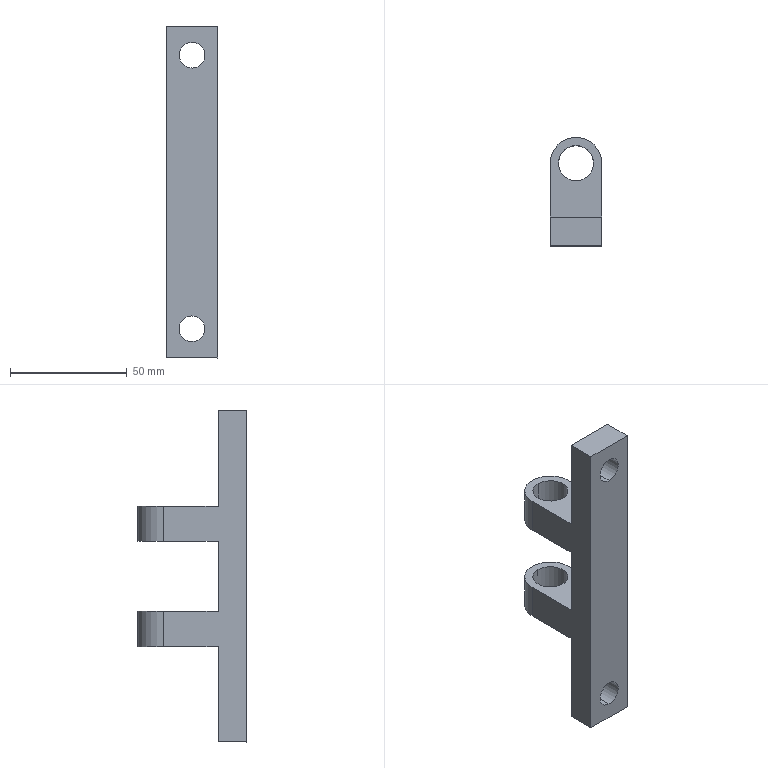Part | SolidWorks | features BaseBody 1 | 1 solid | 22 faces | box 22.041 x 46.517 x 142.008 mm | volume 51119 mm3 | plane 12 | cylinder 10 | commonest cylinder face diameters 11 x4 15 x4 22 x2
STEP:
#1=CARTESIAN_POINT('',(406.066,-39.21,30.764));
#2=VERTEX_POINT('',#1);
#3=CARTESIAN_POINT('',(406.062,-39.209,19.764));
#4=VERTEX_POINT('',#3);
#5=CARTESIAN_POINT('',(406.064,-39.21,25.264));
#6=DIRECTION('',(-0.000000041,-1.,-0.0001428));
#7=DIRECTION('',(-0.0001431,0.0001428,-1.));
#8=AXIS2_PLACEMENT_3D('',#5,#6,#7);
#9=CIRCLE('',#8,5.5);
#10=EDGE_CURVE('',#2,#4,#9,.T.);
#11=ORIENTED_EDGE('',*,*,#10,.F.);
#12=CARTESIAN_POINT('',(406.066,-51.21,30.763));
#13=VERTEX_POINT('',#12);
#14=CARTESIAN_POINT('',(406.066,-51.212,30.763));
#15=DIRECTION('',(-0.000000041,-1.,-0.0001428));
#16=VECTOR('',#15,1000.);
#17=LINE('',#14,#16);
#18=EDGE_CURVE('',#2,#13,#17,.T.);
#19=ORIENTED_EDGE('',*,*,#18,.T.);
#20=CARTESIAN_POINT('',(406.062,-51.209,19.763));
#21=VERTEX_POINT('',#20);
#22=CARTESIAN_POINT('',(406.064,-51.21,25.263));
#23=DIRECTION('',(0.000000041,1.,0.0001428));
#24=DIRECTION('',(-0.0002857,0.0001428,-1.));
#25=AXIS2_PLACEMENT_3D('',#22,#23,#24);
#26=CIRCLE('',#25,5.5);
#27=EDGE_CURVE('',#21,#13,#26,.T.);
#28=ORIENTED_EDGE('',*,*,#27,.F.);
#29=CARTESIAN_POINT('',(406.062,-51.21,19.763));
#30=DIRECTION('',(-0.000000041,-1.,-0.0001428));
#31=VECTOR('',#30,1000.);
#32=LINE('',#29,#31);
#33=EDGE_CURVE('',#4,#21,#32,.T.);
#34=ORIENTED_EDGE('',*,*,#33,.F.);
#35=EDGE_LOOP('',(#11,#19,#28,#34));
#36=FACE_OUTER_BOUND('',#35,.T.);
#37=CARTESIAN_POINT('',(406.064,-51.211,25.263));
#38=DIRECTION('',(-0.000000041,-1.,-0.0001428));
#39=DIRECTION('',(-0.0002857,0.0001428,-1.));
#40=AXIS2_PLACEMENT_3D('',#37,#38,#39);
#41=CYLINDRICAL_SURFACE('',#40,5.5);
#42=ADVANCED_FACE('',(#36),#41,.F.);
#43=CARTESIAN_POINT('',(406.069,-8.211,53.586));
#44=VERTEX_POINT('',#43);
#45=CARTESIAN_POINT('',(406.069,-23.211,53.584));
#46=VERTEX_POINT('',#45);
#47=CARTESIAN_POINT('',(406.069,-15.711,53.585));
#48=DIRECTION('',(0.0002857,-0.0001428,1.));
#49=DIRECTION('',(-0.000000041,-1.,-0.0001428));
#50=AXIS2_PLACEMENT_3D('',#47,#48,#49);
#51=CIRCLE('',#50,7.5);
#52=EDGE_CURVE('',#44,#46,#51,.T.);
#53=ORIENTED_EDGE('',*,*,#52,.F.);
#54=CARTESIAN_POINT('',(406.073,-8.213,68.586));
#55=VERTEX_POINT('',#54);
#56=CARTESIAN_POINT('',(406.069,-8.211,53.586));
#57=DIRECTION('',(0.0002857,-0.0001428,1.));
#58=VECTOR('',#57,1000.);
#59=LINE('',#56,#58);
#60=EDGE_CURVE('',#44,#55,#59,.T.);
#61=ORIENTED_EDGE('',*,*,#60,.T.);
#62=CARTESIAN_POINT('',(406.073,-23.213,68.584));
#63=VERTEX_POINT('',#62);
#64=CARTESIAN_POINT('',(406.073,-15.713,68.585));
#65=DIRECTION('',(-0.0002857,0.0001428,-1.));
#66=DIRECTION('',(-0.000000041,-1.,-0.0001428));
#67=AXIS2_PLACEMENT_3D('',#64,#65,#66);
#68=CIRCLE('',#67,7.5);
#69=EDGE_CURVE('',#63,#55,#68,.T.);
#70=ORIENTED_EDGE('',*,*,#69,.F.);
#71=CARTESIAN_POINT('',(406.069,-23.211,53.584));
#72=DIRECTION('',(0.0002857,-0.0001428,1.));
#73=VECTOR('',#72,1000.);
#74=LINE('',#71,#73);
#75=EDGE_CURVE('',#46,#63,#74,.T.);
#76=ORIENTED_EDGE('',*,*,#75,.F.);
#77=EDGE_LOOP('',(#53,#61,#70,#76));
#78=FACE_OUTER_BOUND('',#77,.T.);
#79=CARTESIAN_POINT('',(406.069,-15.711,53.585));
#80=DIRECTION('',(0.0002857,-0.0001428,1.));
#81=DIRECTION('',(-0.000000041,-1.,-0.0001428));
#82=AXIS2_PLACEMENT_3D('',#79,#80,#81);
#83=CYLINDRICAL_SURFACE('',#82,7.5);
#84=ADVANCED_FACE('',(#78),#83,.F.);
#85=CARTESIAN_POINT('',(406.082,-8.218,98.586));
#86=VERTEX_POINT('',#85);
#87=CARTESIAN_POINT('',(406.082,-23.218,98.584));
#88=VERTEX_POINT('',#87);
#89=CARTESIAN_POINT('',(406.082,-15.718,98.585));
#90=DIRECTION('',(0.0002857,-0.0001428,1.));
#91=DIRECTION('',(0.000000041,1.,0.0001428));
#92=AXIS2_PLACEMENT_3D('',#89,#90,#91);
#93=CIRCLE('',#92,7.5);
#94=EDGE_CURVE('',#86,#88,#93,.T.);
#95=ORIENTED_EDGE('',*,*,#94,.F.);
#96=CARTESIAN_POINT('',(406.086,-8.22,113.586));
#97=VERTEX_POINT('',#96);
#98=CARTESIAN_POINT('',(406.069,-8.211,53.586));
#99=DIRECTION('',(0.0002857,-0.0001428,1.));
#100=VECTOR('',#99,1000.);
#101=LINE('',#98,#100);
#102=EDGE_CURVE('',#86,#97,#101,.T.);
#103=ORIENTED_EDGE('',*,*,#102,.T.);
#104=CARTESIAN_POINT('',(406.086,-23.22,113.584));
#105=VERTEX_POINT('',#104);
#106=CARTESIAN_POINT('',(406.086,-15.72,113.585));
#107=DIRECTION('',(-0.0002857,0.0001428,-1.));
#108=DIRECTION('',(0.000000041,1.,0.0001428));
#109=AXIS2_PLACEMENT_3D('',#106,#107,#108);
#110=CIRCLE('',#109,7.5);
#111=EDGE_CURVE('',#105,#97,#110,.T.);
#112=ORIENTED_EDGE('',*,*,#111,.F.);
#113=CARTESIAN_POINT('',(406.069,-23.211,53.584));
#114=DIRECTION('',(0.0002857,-0.0001428,1.));
#115=VECTOR('',#114,1000.);
#116=LINE('',#113,#115);
#117=EDGE_CURVE('',#88,#105,#116,.T.);
#118=ORIENTED_EDGE('',*,*,#117,.F.);
#119=EDGE_LOOP('',(#95,#103,#112,#118));
#120=FACE_OUTER_BOUND('',#119,.T.);
#121=CARTESIAN_POINT('',(406.069,-15.711,53.585));
#122=DIRECTION('',(0.0002857,-0.0001428,1.));
#123=DIRECTION('',(-0.000000041,-1.,-0.0001428));
#124=AXIS2_PLACEMENT_3D('',#121,#122,#123);
#125=CYLINDRICAL_SURFACE('',#124,7.5);
#126=ADVANCED_FACE('',(#120),#125,.F.);
#127=CARTESIAN_POINT('',(406.093,-39.227,147.764));
#128=VERTEX_POINT('',#127);
#129=CARTESIAN_POINT('',(406.089,-39.226,136.764));
#130=VERTEX_POINT('',#129);
#131=CARTESIAN_POINT('',(406.091,-39.226,142.264));
#132=DIRECTION('',(-0.000000041,-1.,-0.0001428));
#133=DIRECTION('',(-0.0001431,0.0001428,-1.));
#134=AXIS2_PLACEMENT_3D('',#131,#132,#133);
#135=CIRCLE('',#134,5.5);
#136=EDGE_CURVE('',#128,#130,#135,.T.);
#137=ORIENTED_EDGE('',*,*,#136,.F.);
#138=CARTESIAN_POINT('',(406.093,-51.227,147.763));
#139=VERTEX_POINT('',#138);
#140=CARTESIAN_POINT('',(406.093,-51.226,147.763));
#141=DIRECTION('',(-0.000000041,-1.,-0.0001428));
#142=VECTOR('',#141,1000.);
#143=LINE('',#140,#142);
#144=EDGE_CURVE('',#128,#139,#143,.T.);
#145=ORIENTED_EDGE('',*,*,#144,.T.);
#146=CARTESIAN_POINT('',(406.089,-51.226,136.763));
#147=VERTEX_POINT('',#146);
#148=CARTESIAN_POINT('',(406.091,-51.226,142.263));
#149=DIRECTION('',(0.000000041,1.,0.0001428));
#150=DIRECTION('',(-0.0002857,0.0001428,-1.));
#151=AXIS2_PLACEMENT_3D('',#148,#149,#150);
#152=CIRCLE('',#151,5.5);
#153=EDGE_CURVE('',#147,#139,#152,.T.);
#154=ORIENTED_EDGE('',*,*,#153,.F.);
#155=CARTESIAN_POINT('',(406.089,-51.224,136.763));
#156=DIRECTION('',(-0.000000041,-1.,-0.0001428));
#157=VECTOR('',#156,1000.);
#158=LINE('',#155,#157);
#159=EDGE_CURVE('',#130,#147,#158,.T.);
#160=ORIENTED_EDGE('',*,*,#159,.F.);
#161=EDGE_LOOP('',(#137,#145,#154,#160));
#162=FACE_OUTER_BOUND('',#161,.T.);
#163=CARTESIAN_POINT('',(406.091,-51.225,142.263));
#164=DIRECTION('',(-0.000000041,-1.,-0.0001428));
#165=DIRECTION('',(-0.0002857,0.0001428,-1.));
#166=AXIS2_PLACEMENT_3D('',#163,#164,#165);
#167=CYLINDRICAL_SURFACE('',#166,5.5);
#168=ADVANCED_FACE('',(#162),#167,.F.);
#169=CARTESIAN_POINT('',(417.057,-51.208,12.76));
#170=VERTEX_POINT('',#169);
#171=CARTESIAN_POINT('',(417.057,-39.208,12.761));
#172=VERTEX_POINT('',#171);
#173=CARTESIAN_POINT('',(417.057,-51.208,12.76));
#174=DIRECTION('',(0.000000041,1.,0.0001428));
#175=VECTOR('',#174,1000.);
#176=LINE('',#173,#175);
#177=EDGE_CURVE('',#170,#172,#176,.T.);
#178=ORIENTED_EDGE('',*,*,#177,.F.);
#179=CARTESIAN_POINT('',(395.057,-51.208,12.766));
#180=VERTEX_POINT('',#179);
#181=CARTESIAN_POINT('',(395.057,-51.208,12.766));
#182=DIRECTION('',(1.,0.,-0.0002857));
#183=VECTOR('',#182,1000.);
#184=LINE('',#181,#183);
#185=EDGE_CURVE('',#180,#170,#184,.T.);
#186=ORIENTED_EDGE('',*,*,#185,.F.);
#187=CARTESIAN_POINT('',(395.057,-39.208,12.768));
#188=VERTEX_POINT('',#187);
#189=CARTESIAN_POINT('',(395.057,-39.208,12.768));
#190=DIRECTION('',(-0.000000041,-1.,-0.0001428));
#191=VECTOR('',#190,1000.);
#192=LINE('',#189,#191);
#193=EDGE_CURVE('',#188,#180,#192,.T.);
#194=ORIENTED_EDGE('',*,*,#193,.F.);
#195=CARTESIAN_POINT('',(395.057,-39.208,12.768));
#196=DIRECTION('',(1.,0.,-0.0002857));
#197=VECTOR('',#196,1000.);
#198=LINE('',#195,#197);
#199=EDGE_CURVE('',#188,#172,#198,.T.);
#200=ORIENTED_EDGE('',*,*,#199,.T.);
#201=EDGE_LOOP('',(#178,#186,#194,#200));
#202=FACE_OUTER_BOUND('',#201,.T.);
#203=CARTESIAN_POINT('',(406.06,-51.209,12.763));
#204=DIRECTION('',(0.0002857,-0.0001428,1.));
#205=DIRECTION('',(-0.4472,-0.8944,0.));
#206=AXIS2_PLACEMENT_3D('',#203,#204,#205);
#207=PLANE('',#206);
#208=ADVANCED_FACE('',(#202),#207,.F.);
#209=ORIENTED_EDGE('',*,*,#144,.F.);
#210=CARTESIAN_POINT('',(406.091,-39.226,142.264));
#211=DIRECTION('',(-0.000000041,-1.,-0.0001428));
#212=DIRECTION('',(-0.0001431,0.0001428,-1.));
#213=AXIS2_PLACEMENT_3D('',#210,#211,#212);
#214=CIRCLE('',#213,5.5);
#215=EDGE_CURVE('',#130,#128,#214,.T.);
#216=ORIENTED_EDGE('',*,*,#215,.F.);
#217=ORIENTED_EDGE('',*,*,#159,.T.);
#218=CARTESIAN_POINT('',(406.091,-51.226,142.263));
#219=DIRECTION('',(0.000000041,1.,0.0001428));
#220=DIRECTION('',(-0.0002857,0.0001428,-1.));
#221=AXIS2_PLACEMENT_3D('',#218,#219,#220);
#222=CIRCLE('',#221,5.5);
#223=EDGE_CURVE('',#139,#147,#222,.T.);
#224=ORIENTED_EDGE('',*,*,#223,.F.);
#225=EDGE_LOOP('',(#209,#216,#217,#224));
#226=FACE_OUTER_BOUND('',#225,.T.);
#227=CARTESIAN_POINT('',(406.091,-51.225,142.263));
#228=DIRECTION('',(-0.000000041,-1.,-0.0001428));
#229=DIRECTION('',(-0.0002857,0.0001428,-1.));
#230=AXIS2_PLACEMENT_3D('',#227,#228,#229);
#231=CYLINDRICAL_SURFACE('',#230,5.5);
#232=ADVANCED_FACE('',(#226),#231,.F.);
#233=ORIENTED_EDGE('',*,*,#215,.T.);
#234=ORIENTED_EDGE('',*,*,#136,.T.);
#235=EDGE_LOOP('',(#233,#234));
#236=FACE_BOUND('',#235,.T.);
#237=CARTESIAN_POINT('',(417.098,-39.228,154.761));
#238=VERTEX_POINT('',#237);
#239=CARTESIAN_POINT('',(417.086,-39.222,113.579));
#240=VERTEX_POINT('',#239);
#241=CARTESIAN_POINT('',(417.098,-39.228,154.761));
#242=DIRECTION('',(-0.0002857,0.0001428,-1.));
#243=VECTOR('',#242,1000.);
#244=LINE('',#241,#243);
#245=EDGE_CURVE('',#238,#240,#244,.T.);
#246=ORIENTED_EDGE('',*,*,#245,.T.);
#247=CARTESIAN_POINT('',(395.086,-39.222,113.585));
#248=VERTEX_POINT('',#247);
#249=CARTESIAN_POINT('',(417.086,-39.222,113.579));
#250=DIRECTION('',(-1.,0.,0.0002857));
#251=VECTOR('',#250,1000.);
#252=LINE('',#249,#251);
#253=EDGE_CURVE('',#240,#248,#252,.T.);
#254=ORIENTED_EDGE('',*,*,#253,.T.);
#255=CARTESIAN_POINT('',(395.098,-39.228,154.768));
#256=VERTEX_POINT('',#255);
#257=CARTESIAN_POINT('',(395.086,-39.222,113.585));
#258=DIRECTION('',(0.0002857,-0.0001428,1.));
#259=VECTOR('',#258,1000.);
#260=LINE('',#257,#259);
#261=EDGE_CURVE('',#248,#256,#260,.T.);
#262=ORIENTED_EDGE('',*,*,#261,.T.);
#263=CARTESIAN_POINT('',(417.098,-39.228,154.761));
#264=DIRECTION('',(-1.,0.,0.0002857));
#265=VECTOR('',#264,1000.);
#266=LINE('',#263,#265);
#267=EDGE_CURVE('',#238,#256,#266,.T.);
#268=ORIENTED_EDGE('',*,*,#267,.F.);
#269=EDGE_LOOP('',(#246,#254,#262,#268));
#270=FACE_OUTER_BOUND('',#269,.T.);
#271=CARTESIAN_POINT('',(406.078,-39.218,83.764));
#272=DIRECTION('',(0.000000041,1.,0.0001428));
#273=DIRECTION('',(1.,0.,-0.0002857));
#274=AXIS2_PLACEMENT_3D('',#271,#272,#273);
#275=PLANE('',#274);
#276=ADVANCED_FACE('',(#236,#270),#275,.T.);
#277=CARTESIAN_POINT('',(417.082,-39.22,98.579));
#278=VERTEX_POINT('',#277);
#279=CARTESIAN_POINT('',(417.073,-39.216,68.579));
#280=VERTEX_POINT('',#279);
#281=CARTESIAN_POINT('',(417.082,-39.22,98.579));
#282=DIRECTION('',(-0.0002857,0.0001428,-1.));
#283=VECTOR('',#282,1000.);
#284=LINE('',#281,#283);
#285=EDGE_CURVE('',#278,#280,#284,.T.);
#286=ORIENTED_EDGE('',*,*,#285,.T.);
#287=CARTESIAN_POINT('',(395.073,-39.216,68.585));
#288=VERTEX_POINT('',#287);
#289=CARTESIAN_POINT('',(395.073,-39.216,68.585));
#290=DIRECTION('',(1.,0.,-0.0002857));
#291=VECTOR('',#290,1000.);
#292=LINE('',#289,#291);
#293=EDGE_CURVE('',#288,#280,#292,.T.);
#294=ORIENTED_EDGE('',*,*,#293,.F.);
#295=CARTESIAN_POINT('',(395.082,-39.22,98.585));
#296=VERTEX_POINT('',#295);
#297=CARTESIAN_POINT('',(395.073,-39.216,68.585));
#298=DIRECTION('',(0.0002857,-0.0001428,1.));
#299=VECTOR('',#298,1000.);
#300=LINE('',#297,#299);
#301=EDGE_CURVE('',#288,#296,#300,.T.);
#302=ORIENTED_EDGE('',*,*,#301,.T.);
#303=CARTESIAN_POINT('',(417.082,-39.22,98.579));
#304=DIRECTION('',(-1.,0.,0.0002857));
#305=VECTOR('',#304,1000.);
#306=LINE('',#303,#305);
#307=EDGE_CURVE('',#278,#296,#306,.T.);
#308=ORIENTED_EDGE('',*,*,#307,.F.);
#309=EDGE_LOOP('',(#286,#294,#302,#308));
#310=FACE_OUTER_BOUND('',#309,.T.);
#311=CARTESIAN_POINT('',(406.078,-39.218,83.764));
#312=DIRECTION('',(0.000000041,1.,0.0001428));
#313=DIRECTION('',(1.,0.,-0.0002857));
#314=AXIS2_PLACEMENT_3D('',#311,#312,#313);
#315=PLANE('',#314);
#316=ADVANCED_FACE('',(#310),#315,.T.);
#317=CARTESIAN_POINT('',(395.069,-15.711,53.588));
#318=VERTEX_POINT('',#317);
#319=CARTESIAN_POINT('',(395.073,-15.713,68.588));
#320=VERTEX_POINT('',#319);
#321=CARTESIAN_POINT('',(395.069,-15.711,53.588));
#322=DIRECTION('',(0.0002857,-0.0001428,1.));
#323=VECTOR('',#322,1000.);
#324=LINE('',#321,#323);
#325=EDGE_CURVE('',#318,#320,#324,.T.);
#326=ORIENTED_EDGE('',*,*,#325,.F.);
#327=CARTESIAN_POINT('',(395.069,-39.214,53.585));
#328=VERTEX_POINT('',#327);
#329=CARTESIAN_POINT('',(395.069,-39.214,53.585));
#330=DIRECTION('',(0.000000041,1.,0.0001428));
#331=VECTOR('',#330,1000.);
#332=LINE('',#329,#331);
#333=EDGE_CURVE('',#328,#318,#332,.T.);
#334=ORIENTED_EDGE('',*,*,#333,.F.);
#335=CARTESIAN_POINT('',(395.057,-39.208,12.768));
#336=DIRECTION('',(0.0002857,-0.0001428,1.));
#337=VECTOR('',#336,1000.);
#338=LINE('',#335,#337);
#339=EDGE_CURVE('',#188,#328,#338,.T.);
#340=ORIENTED_EDGE('',*,*,#339,.F.);
#341=ORIENTED_EDGE('',*,*,#193,.T.);
#342=CARTESIAN_POINT('',(395.098,-51.228,154.766));
#343=VERTEX_POINT('',#342);
#344=CARTESIAN_POINT('',(395.098,-51.228,154.766));
#345=DIRECTION('',(-0.0002857,0.0001428,-1.));
#346=VECTOR('',#345,1000.);
#347=LINE('',#344,#346);
#348=EDGE_CURVE('',#343,#180,#347,.T.);
#349=ORIENTED_EDGE('',*,*,#348,.F.);
#350=CARTESIAN_POINT('',(395.098,-51.228,154.766));
#351=DIRECTION('',(0.000000041,1.,0.0001428));
#352=VECTOR('',#351,1000.);
#353=LINE('',#350,#352);
#354=EDGE_CURVE('',#343,#256,#353,.T.);
#355=ORIENTED_EDGE('',*,*,#354,.T.);
#356=ORIENTED_EDGE('',*,*,#261,.F.);
#357=CARTESIAN_POINT('',(395.086,-15.72,113.588));
#358=VERTEX_POINT('',#357);
#359=CARTESIAN_POINT('',(395.086,-39.222,113.585));
#360=DIRECTION('',(0.000000041,1.,0.0001428));
#361=VECTOR('',#360,1000.);
#362=LINE('',#359,#361);
#363=EDGE_CURVE('',#248,#358,#362,.T.);
#364=ORIENTED_EDGE('',*,*,#363,.T.);
#365=CARTESIAN_POINT('',(395.082,-15.718,98.588));
#366=VERTEX_POINT('',#365);
#367=CARTESIAN_POINT('',(395.082,-15.718,98.588));
#368=DIRECTION('',(0.0002857,-0.0001428,1.));
#369=VECTOR('',#368,1000.);
#370=LINE('',#367,#369);
#371=EDGE_CURVE('',#366,#358,#370,.T.);
#372=ORIENTED_EDGE('',*,*,#371,.F.);
#373=CARTESIAN_POINT('',(395.082,-39.22,98.585));
#374=DIRECTION('',(0.000000041,1.,0.0001428));
#375=VECTOR('',#374,1000.);
#376=LINE('',#373,#375);
#377=EDGE_CURVE('',#296,#366,#376,.T.);
#378=ORIENTED_EDGE('',*,*,#377,.F.);
#379=ORIENTED_EDGE('',*,*,#301,.F.);
#380=CARTESIAN_POINT('',(395.073,-39.216,68.585));
#381=DIRECTION('',(0.000000041,1.,0.0001428));
#382=VECTOR('',#381,1000.);
#383=LINE('',#380,#382);
#384=EDGE_CURVE('',#288,#320,#383,.T.);
#385=ORIENTED_EDGE('',*,*,#384,.T.);
#386=EDGE_LOOP('',(#326,#334,#340,#341,#349,#355,#356,#364,#372,#378,#379,#385));
#387=FACE_OUTER_BOUND('',#386,.T.);
#388=CARTESIAN_POINT('',(395.077,4.285,83.591));
#389=DIRECTION('',(-1.,0.,0.0002857));
#390=DIRECTION('',(0.,1.,0.));
#391=AXIS2_PLACEMENT_3D('',#388,#389,#390);
#392=PLANE('',#391);
#393=ADVANCED_FACE('',(#387),#392,.T.);
#394=CARTESIAN_POINT('',(417.082,-15.718,98.582));
#395=VERTEX_POINT('',#394);
#396=CARTESIAN_POINT('',(406.082,-15.718,98.585));
#397=DIRECTION('',(-0.0002857,0.0001428,-1.));
#398=DIRECTION('',(-1.,0.,0.0002857));
#399=AXIS2_PLACEMENT_3D('',#396,#397,#398);
#400=CIRCLE('',#399,11.);
#401=EDGE_CURVE('',#366,#395,#400,.T.);
#402=ORIENTED_EDGE('',*,*,#401,.F.);
#403=ORIENTED_EDGE('',*,*,#371,.T.);
#404=CARTESIAN_POINT('',(417.086,-15.72,113.582));
#405=VERTEX_POINT('',#404);
#406=CARTESIAN_POINT('',(406.086,-15.72,113.585));
#407=DIRECTION('',(0.0002857,-0.0001428,1.));
#408=DIRECTION('',(0.000000041,1.,0.0001428));
#409=AXIS2_PLACEMENT_3D('',#406,#407,#408);
#410=CIRCLE('',#409,11.);
#411=EDGE_CURVE('',#405,#358,#410,.T.);
#412=ORIENTED_EDGE('',*,*,#411,.F.);
#413=CARTESIAN_POINT('',(417.086,-15.72,113.582));
#414=DIRECTION('',(-0.0002857,0.0001428,-1.));
#415=VECTOR('',#414,1000.);
#416=LINE('',#413,#415);
#417=EDGE_CURVE('',#405,#395,#416,.T.);
#418=ORIENTED_EDGE('',*,*,#417,.T.);
#419=EDGE_LOOP('',(#402,#403,#412,#418));
#420=FACE_OUTER_BOUND('',#419,.T.);
#421=CARTESIAN_POINT('',(406.077,-15.715,83.585));
#422=DIRECTION('',(0.0002857,-0.0001428,1.));
#423=DIRECTION('',(-0.000000041,-1.,-0.0001428));
#424=AXIS2_PLACEMENT_3D('',#421,#422,#423);
#425=CYLINDRICAL_SURFACE('',#424,11.);
#426=ADVANCED_FACE('',(#420),#425,.T.);
#427=ORIENTED_EDGE('',*,*,#111,.T.);
#428=CARTESIAN_POINT('',(406.086,-15.72,113.585));
#429=DIRECTION('',(-0.0002857,0.0001428,-1.));
#430=DIRECTION('',(0.000000041,1.,0.0001428));
#431=AXIS2_PLACEMENT_3D('',#428,#429,#430);
#432=CIRCLE('',#431,7.5);
#433=EDGE_CURVE('',#97,#105,#432,.T.);
#434=ORIENTED_EDGE('',*,*,#433,.T.);
#435=EDGE_LOOP('',(#427,#434));
#436=FACE_BOUND('',#435,.T.);
#437=ORIENTED_EDGE('',*,*,#411,.T.);
#438=ORIENTED_EDGE('',*,*,#363,.F.);
#439=ORIENTED_EDGE('',*,*,#253,.F.);
#440=CARTESIAN_POINT('',(417.086,-39.222,113.579));
#441=DIRECTION('',(0.000000041,1.,0.0001428));
#442=VECTOR('',#441,1000.);
#443=LINE('',#440,#442);
#444=EDGE_CURVE('',#240,#405,#443,.T.);
#445=ORIENTED_EDGE('',*,*,#444,.T.);
#446=EDGE_LOOP('',(#437,#438,#439,#445));
#447=FACE_OUTER_BOUND('',#446,.T.);
#448=CARTESIAN_POINT('',(406.086,4.28,113.588));
#449=DIRECTION('',(0.0002857,-0.0001428,1.));
#450=DIRECTION('',(-0.4472,-0.8944,0.));
#451=AXIS2_PLACEMENT_3D('',#448,#449,#450);
#452=PLANE('',#451);
#453=ADVANCED_FACE('',(#436,#447),#452,.T.);
#454=ORIENTED_EDGE('',*,*,#102,.F.);
#455=CARTESIAN_POINT('',(406.082,-15.718,98.585));
#456=DIRECTION('',(0.0002857,-0.0001428,1.));
#457=DIRECTION('',(0.000000041,1.,0.0001428));
#458=AXIS2_PLACEMENT_3D('',#455,#456,#457);
#459=CIRCLE('',#458,7.5);
#460=EDGE_CURVE('',#88,#86,#459,.T.);
#461=ORIENTED_EDGE('',*,*,#460,.F.);
#462=ORIENTED_EDGE('',*,*,#117,.T.);
#463=ORIENTED_EDGE('',*,*,#433,.F.);
#464=EDGE_LOOP('',(#454,#461,#462,#463));
#465=FACE_OUTER_BOUND('',#464,.T.);
#466=CARTESIAN_POINT('',(406.069,-15.711,53.585));
#467=DIRECTION('',(0.0002857,-0.0001428,1.));
#468=DIRECTION('',(-0.000000041,-1.,-0.0001428));
#469=AXIS2_PLACEMENT_3D('',#466,#467,#468);
#470=CYLINDRICAL_SURFACE('',#469,7.5);
#471=ADVANCED_FACE('',(#465),#470,.F.);
#472=ORIENTED_EDGE('',*,*,#460,.T.);
#473=ORIENTED_EDGE('',*,*,#94,.T.);
#474=EDGE_LOOP('',(#472,#473));
#475=FACE_BOUND('',#474,.T.);
#476=ORIENTED_EDGE('',*,*,#401,.T.);
#477=CARTESIAN_POINT('',(417.082,-39.22,98.579));
#478=DIRECTION('',(0.000000041,1.,0.0001428));
#479=VECTOR('',#478,1000.);
#480=LINE('',#477,#479);
#481=EDGE_CURVE('',#278,#395,#480,.T.);
#482=ORIENTED_EDGE('',*,*,#481,.F.);
#483=ORIENTED_EDGE('',*,*,#307,.T.);
#484=ORIENTED_EDGE('',*,*,#377,.T.);
#485=EDGE_LOOP('',(#476,#482,#483,#484));
#486=FACE_OUTER_BOUND('',#485,.T.);
#487=CARTESIAN_POINT('',(406.082,4.282,98.588));
#488=DIRECTION('',(0.0002857,-0.0001428,1.));
#489=DIRECTION('',(-0.4472,-0.8944,0.));
#490=AXIS2_PLACEMENT_3D('',#487,#488,#489);
#491=PLANE('',#490);
#492=ADVANCED_FACE('',(#475,#486),#491,.F.);
#493=ORIENTED_EDGE('',*,*,#417,.F.);
#494=ORIENTED_EDGE('',*,*,#444,.F.);
#495=ORIENTED_EDGE('',*,*,#245,.F.);
#496=CARTESIAN_POINT('',(417.098,-51.228,154.76));
#497=VERTEX_POINT('',#496);
#498=CARTESIAN_POINT('',(417.098,-39.228,154.761));
#499=DIRECTION('',(-0.000000041,-1.,-0.0001428));
#500=VECTOR('',#499,1000.);
#501=LINE('',#498,#500);
#502=EDGE_CURVE('',#238,#497,#501,.T.);
#503=ORIENTED_EDGE('',*,*,#502,.T.);
#504=CARTESIAN_POINT('',(417.057,-51.208,12.76));
#505=DIRECTION('',(0.0002857,-0.0001428,1.));
#506=VECTOR('',#505,1000.);
#507=LINE('',#504,#506);
#508=EDGE_CURVE('',#170,#497,#507,.T.);
#509=ORIENTED_EDGE('',*,*,#508,.F.);
#510=ORIENTED_EDGE('',*,*,#177,.T.);
#511=CARTESIAN_POINT('',(417.069,-39.214,53.579));
#512=VERTEX_POINT('',#511);
#513=CARTESIAN_POINT('',(417.069,-39.214,53.579));
#514=DIRECTION('',(-0.0002857,0.0001428,-1.));
#515=VECTOR('',#514,1000.);
#516=LINE('',#513,#515);
#517=EDGE_CURVE('',#512,#172,#516,.T.);
#518=ORIENTED_EDGE('',*,*,#517,.F.);
#519=CARTESIAN_POINT('',(417.069,-15.711,53.582));
#520=VERTEX_POINT('',#519);
#521=CARTESIAN_POINT('',(417.069,-39.214,53.579));
#522=DIRECTION('',(0.000000041,1.,0.0001428));
#523=VECTOR('',#522,1000.);
#524=LINE('',#521,#523);
#525=EDGE_CURVE('',#512,#520,#524,.T.);
#526=ORIENTED_EDGE('',*,*,#525,.T.);
#527=CARTESIAN_POINT('',(417.073,-15.713,68.582));
#528=VERTEX_POINT('',#527);
#529=CARTESIAN_POINT('',(417.073,-15.713,68.582));
#530=DIRECTION('',(-0.0002857,0.0001428,-1.));
#531=VECTOR('',#530,1000.);
#532=LINE('',#529,#531);
#533=EDGE_CURVE('',#528,#520,#532,.T.);
#534=ORIENTED_EDGE('',*,*,#533,.F.);
#535=CARTESIAN_POINT('',(417.073,-39.216,68.579));
#536=DIRECTION('',(0.000000041,1.,0.0001428));
#537=VECTOR('',#536,1000.);
#538=LINE('',#535,#537);
#539=EDGE_CURVE('',#280,#528,#538,.T.);
#540=ORIENTED_EDGE('',*,*,#539,.F.);
#541=ORIENTED_EDGE('',*,*,#285,.F.);
#542=ORIENTED_EDGE('',*,*,#481,.T.);
#543=EDGE_LOOP('',(#493,#494,#495,#503,#509,#510,#518,#526,#534,#540,#541,#542));
#544=FACE_OUTER_BOUND('',#543,.T.);
#545=CARTESIAN_POINT('',(417.077,4.285,83.585));
#546=DIRECTION('',(1.,0.,-0.0002857));
#547=DIRECTION('',(0.,-1.,0.));
#548=AXIS2_PLACEMENT_3D('',#545,#546,#547);
#549=PLANE('',#548);
#550=ADVANCED_FACE('',(#544),#549,.T.);
#551=ORIENTED_EDGE('',*,*,#325,.T.);
#552=CARTESIAN_POINT('',(406.073,-15.713,68.585));
#553=DIRECTION('',(0.0002857,-0.0001428,1.));
#554=DIRECTION('',(1.,0.,-0.0002857));
#555=AXIS2_PLACEMENT_3D('',#552,#553,#554);
#556=CIRCLE('',#555,11.);
#557=EDGE_CURVE('',#528,#320,#556,.T.);
#558=ORIENTED_EDGE('',*,*,#557,.F.);
#559=ORIENTED_EDGE('',*,*,#533,.T.);
#560=CARTESIAN_POINT('',(406.069,-15.711,53.585));
#561=DIRECTION('',(-0.0002857,0.0001428,-1.));
#562=DIRECTION('',(-1.,0.,0.0002857));
#563=AXIS2_PLACEMENT_3D('',#560,#561,#562);
#564=CIRCLE('',#563,11.);
#565=EDGE_CURVE('',#318,#520,#564,.T.);
#566=ORIENTED_EDGE('',*,*,#565,.F.);
#567=EDGE_LOOP('',(#551,#558,#559,#566));
#568=FACE_OUTER_BOUND('',#567,.T.);
#569=CARTESIAN_POINT('',(406.077,-15.715,83.585));
#570=DIRECTION('',(0.0002857,-0.0001428,1.));
#571=DIRECTION('',(-0.000000041,-1.,-0.0001428));
#572=AXIS2_PLACEMENT_3D('',#569,#570,#571);
#573=CYLINDRICAL_SURFACE('',#572,11.);
#574=ADVANCED_FACE('',(#568),#573,.T.);
#575=ORIENTED_EDGE('',*,*,#69,.T.);
#576=CARTESIAN_POINT('',(406.073,-15.713,68.585));
#577=DIRECTION('',(-0.0002857,0.0001428,-1.));
#578=DIRECTION('',(-0.000000041,-1.,-0.0001428));
#579=AXIS2_PLACEMENT_3D('',#576,#577,#578);
#580=CIRCLE('',#579,7.5);
#581=EDGE_CURVE('',#55,#63,#580,.T.);
#582=ORIENTED_EDGE('',*,*,#581,.T.);
#583=EDGE_LOOP('',(#575,#582));
#584=FACE_BOUND('',#583,.T.);
#585=ORIENTED_EDGE('',*,*,#384,.F.);
#586=ORIENTED_EDGE('',*,*,#293,.T.);
#587=ORIENTED_EDGE('',*,*,#539,.T.);
#588=ORIENTED_EDGE('',*,*,#557,.T.);
#589=EDGE_LOOP('',(#585,#586,#587,#588));
#590=FACE_OUTER_BOUND('',#589,.T.);
#591=CARTESIAN_POINT('',(406.073,4.287,68.588));
#592=DIRECTION('',(-0.0002857,0.0001428,-1.));
#593=DIRECTION('',(-1.,0.,0.0002857));
#594=AXIS2_PLACEMENT_3D('',#591,#592,#593);
#595=PLANE('',#594);
#596=ADVANCED_FACE('',(#584,#590),#595,.F.);
#597=ORIENTED_EDGE('',*,*,#60,.F.);
#598=CARTESIAN_POINT('',(406.069,-15.711,53.585));
#599=DIRECTION('',(0.0002857,-0.0001428,1.));
#600=DIRECTION('',(-0.000000041,-1.,-0.0001428));
#601=AXIS2_PLACEMENT_3D('',#598,#599,#600);
#602=CIRCLE('',#601,7.5);
#603=EDGE_CURVE('',#46,#44,#602,.T.);
#604=ORIENTED_EDGE('',*,*,#603,.F.);
#605=ORIENTED_EDGE('',*,*,#75,.T.);
#606=ORIENTED_EDGE('',*,*,#581,.F.);
#607=EDGE_LOOP('',(#597,#604,#605,#606));
#608=FACE_OUTER_BOUND('',#607,.T.);
#609=CARTESIAN_POINT('',(406.069,-15.711,53.585));
#610=DIRECTION('',(0.0002857,-0.0001428,1.));
#611=DIRECTION('',(-0.000000041,-1.,-0.0001428));
#612=AXIS2_PLACEMENT_3D('',#609,#610,#611);
#613=CYLINDRICAL_SURFACE('',#612,7.5);
#614=ADVANCED_FACE('',(#608),#613,.F.);
#615=ORIENTED_EDGE('',*,*,#603,.T.);
#616=ORIENTED_EDGE('',*,*,#52,.T.);
#617=EDGE_LOOP('',(#615,#616));
#618=FACE_BOUND('',#617,.T.);
#619=ORIENTED_EDGE('',*,*,#565,.T.);
#620=ORIENTED_EDGE('',*,*,#525,.F.);
#621=CARTESIAN_POINT('',(395.069,-39.214,53.585));
#622=DIRECTION('',(1.,0.,-0.0002857));
#623=VECTOR('',#622,1000.);
#624=LINE('',#621,#623);
#625=EDGE_CURVE('',#328,#512,#624,.T.);
#626=ORIENTED_EDGE('',*,*,#625,.F.);
#627=ORIENTED_EDGE('',*,*,#333,.T.);
#628=EDGE_LOOP('',(#619,#620,#626,#627));
#629=FACE_OUTER_BOUND('',#628,.T.);
#630=CARTESIAN_POINT('',(406.069,4.289,53.588));
#631=DIRECTION('',(-0.0002857,0.0001428,-1.));
#632=DIRECTION('',(-1.,0.,0.0002857));
#633=AXIS2_PLACEMENT_3D('',#630,#631,#632);
#634=PLANE('',#633);
#635=ADVANCED_FACE('',(#618,#629),#634,.T.);
#636=CARTESIAN_POINT('',(406.064,-39.21,25.264));
#637=DIRECTION('',(-0.000000041,-1.,-0.0001428));
#638=DIRECTION('',(-0.0001431,0.0001428,-1.));
#639=AXIS2_PLACEMENT_3D('',#636,#637,#638);
#640=CIRCLE('',#639,5.5);
#641=EDGE_CURVE('',#4,#2,#640,.T.);
#642=ORIENTED_EDGE('',*,*,#641,.T.);
#643=ORIENTED_EDGE('',*,*,#10,.T.);
#644=EDGE_LOOP('',(#642,#643));
#645=FACE_BOUND('',#644,.T.);
#646=ORIENTED_EDGE('',*,*,#517,.T.);
#647=ORIENTED_EDGE('',*,*,#199,.F.);
#648=ORIENTED_EDGE('',*,*,#339,.T.);
#649=ORIENTED_EDGE('',*,*,#625,.T.);
#650=EDGE_LOOP('',(#646,#647,#648,#649));
#651=FACE_OUTER_BOUND('',#650,.T.);
#652=CARTESIAN_POINT('',(406.078,-39.218,83.764));
#653=DIRECTION('',(0.000000041,1.,0.0001428));
#654=DIRECTION('',(1.,0.,-0.0002857));
#655=AXIS2_PLACEMENT_3D('',#652,#653,#654);
#656=PLANE('',#655);
#657=ADVANCED_FACE('',(#645,#651),#656,.T.);
#658=ORIENTED_EDGE('',*,*,#18,.F.);
#659=ORIENTED_EDGE('',*,*,#641,.F.);
#660=ORIENTED_EDGE('',*,*,#33,.T.);
#661=CARTESIAN_POINT('',(406.064,-51.21,25.263));
#662=DIRECTION('',(0.000000041,1.,0.0001428));
#663=DIRECTION('',(-0.0002857,0.0001428,-1.));
#664=AXIS2_PLACEMENT_3D('',#661,#662,#663);
#665=CIRCLE('',#664,5.5);
#666=EDGE_CURVE('',#13,#21,#665,.T.);
#667=ORIENTED_EDGE('',*,*,#666,.F.);
#668=EDGE_LOOP('',(#658,#659,#660,#667));
#669=FACE_OUTER_BOUND('',#668,.T.);
#670=CARTESIAN_POINT('',(406.064,-51.211,25.263));
#671=DIRECTION('',(-0.000000041,-1.,-0.0001428));
#672=DIRECTION('',(-0.0002857,0.0001428,-1.));
#673=AXIS2_PLACEMENT_3D('',#670,#671,#672);
#674=CYLINDRICAL_SURFACE('',#673,5.5);
#675=ADVANCED_FACE('',(#669),#674,.F.);
#676=ORIENTED_EDGE('',*,*,#27,.T.);
#677=ORIENTED_EDGE('',*,*,#666,.T.);
#678=EDGE_LOOP('',(#676,#677));
#679=FACE_BOUND('',#678,.T.);
#680=ORIENTED_EDGE('',*,*,#153,.T.);
#681=ORIENTED_EDGE('',*,*,#223,.T.);
#682=EDGE_LOOP('',(#680,#681));
#683=FACE_BOUND('',#682,.T.);
#684=CARTESIAN_POINT('',(417.098,-51.228,154.76));
#685=DIRECTION('',(-1.,0.,0.0002857));
#686=VECTOR('',#685,1000.);
#687=LINE('',#684,#686);
#688=EDGE_CURVE('',#497,#343,#687,.T.);
#689=ORIENTED_EDGE('',*,*,#688,.T.);
#690=ORIENTED_EDGE('',*,*,#348,.T.);
#691=ORIENTED_EDGE('',*,*,#185,.T.);
#692=ORIENTED_EDGE('',*,*,#508,.T.);
#693=EDGE_LOOP('',(#689,#690,#691,#692));
#694=FACE_OUTER_BOUND('',#693,.T.);
#695=CARTESIAN_POINT('',(406.078,-51.218,83.763));
#696=DIRECTION('',(0.000000041,1.,0.0001428));
#697=DIRECTION('',(1.,0.,-0.0002857));
#698=AXIS2_PLACEMENT_3D('',#695,#696,#697);
#699=PLANE('',#698);
#700=ADVANCED_FACE('',(#679,#683,#694),#699,.F.);
#701=ORIENTED_EDGE('',*,*,#502,.F.);
#702=ORIENTED_EDGE('',*,*,#267,.T.);
#703=ORIENTED_EDGE('',*,*,#354,.F.);
#704=ORIENTED_EDGE('',*,*,#688,.F.);
#705=EDGE_LOOP('',(#701,#702,#703,#704));
#706=FACE_OUTER_BOUND('',#705,.T.);
#707=CARTESIAN_POINT('',(406.095,-51.227,154.763));
#708=DIRECTION('',(0.0002857,-0.0001428,1.));
#709=DIRECTION('',(-0.4472,-0.8944,0.));
#710=AXIS2_PLACEMENT_3D('',#707,#708,#709);
#711=PLANE('',#710);
#712=ADVANCED_FACE('',(#706),#711,.T.);
#713=CLOSED_SHELL('',(#42,#84,#126,#168,#208,#232,#276,#316,#393,#426,#453,#471,#492,#550,#574,#596,#614,#635,#657,#675,#700,#712));
#714=MANIFOLD_SOLID_BREP('',#713);
#715=CARTESIAN_POINT('',(0.,0.,0.));
#716=DIRECTION('',(0.,0.,1.));
#717=DIRECTION('',(1.,0.,0.));
#718=AXIS2_PLACEMENT_3D('',#715,#716,#717);
#719=(LENGTH_UNIT()NAMED_UNIT(*)SI_UNIT(.MILLI.,.METRE.));
#720=UNCERTAINTY_MEASURE_WITH_UNIT(LENGTH_MEASURE(0.00001),#719,'','');
#721=(NAMED_UNIT(*)PLANE_ANGLE_UNIT()SI_UNIT($,.RADIAN.));
#722=(NAMED_UNIT(*)SI_UNIT($,.STERADIAN.)SOLID_ANGLE_UNIT());
#723=(GEOMETRIC_REPRESENTATION_CONTEXT(3)GLOBAL_UNCERTAINTY_ASSIGNED_CONTEXT((#720))GLOBAL_UNIT_ASSIGNED_CONTEXT((#719,#721,#722))REPRESENTATION_CONTEXT('',''));
#724=ADVANCED_BREP_SHAPE_REPRESENTATION('',(#714,#718),#723);